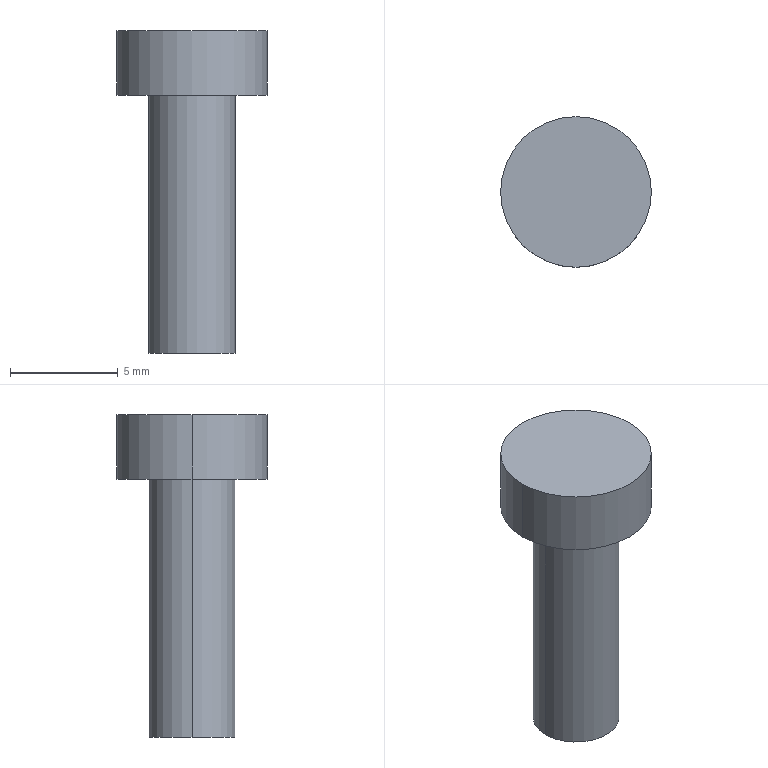Part | SolidWorks | features Extrusion 1, ICE 1 | 1 solid | 7 faces | box 7 x 7 x 15 mm | volume 266.25 mm3 | cylinder 4 | plane 3 | commonest cylinder face diameters 4 x2 7 x2
STEP:
#1=CARTESIAN_POINT('',(3.5,0.,3.));
#2=VERTEX_POINT('',#1);
#3=CARTESIAN_POINT('',(-3.5,0.,3.));
#4=VERTEX_POINT('',#3);
#5=CARTESIAN_POINT('',(0.,0.,3.));
#6=DIRECTION('',(0.,0.,1.));
#7=DIRECTION('',(1.,0.,0.));
#8=AXIS2_PLACEMENT_3D('',#5,#6,#7);
#9=CIRCLE('',#8,3.5);
#10=EDGE_CURVE('',#2,#4,#9,.T.);
#11=ORIENTED_EDGE('',*,*,#10,.F.);
#12=CARTESIAN_POINT('',(3.5,0.,0.));
#13=VERTEX_POINT('',#12);
#14=CARTESIAN_POINT('',(3.5,0.,3.));
#15=DIRECTION('',(0.,0.,-1.));
#16=VECTOR('',#15,1000.);
#17=LINE('',#14,#16);
#18=EDGE_CURVE('',#2,#13,#17,.T.);
#19=ORIENTED_EDGE('',*,*,#18,.T.);
#20=CARTESIAN_POINT('',(-3.5,0.,0.));
#21=VERTEX_POINT('',#20);
#22=CARTESIAN_POINT('',(0.,0.,0.));
#23=DIRECTION('',(0.,0.,1.));
#24=DIRECTION('',(1.,0.,0.));
#25=AXIS2_PLACEMENT_3D('',#22,#23,#24);
#26=CIRCLE('',#25,3.5);
#27=EDGE_CURVE('',#13,#21,#26,.T.);
#28=ORIENTED_EDGE('',*,*,#27,.T.);
#29=CARTESIAN_POINT('',(-3.5,0.,3.));
#30=DIRECTION('',(0.,0.,-1.));
#31=VECTOR('',#30,1000.);
#32=LINE('',#29,#31);
#33=EDGE_CURVE('',#4,#21,#32,.T.);
#34=ORIENTED_EDGE('',*,*,#33,.F.);
#35=EDGE_LOOP('',(#11,#19,#28,#34));
#36=FACE_OUTER_BOUND('',#35,.T.);
#37=CARTESIAN_POINT('',(0.,0.,3.));
#38=DIRECTION('',(0.,0.,-1.));
#39=DIRECTION('',(-1.,0.,0.));
#40=AXIS2_PLACEMENT_3D('',#37,#38,#39);
#41=CYLINDRICAL_SURFACE('',#40,3.5);
#42=ADVANCED_FACE('',(#36),#41,.T.);
#43=CARTESIAN_POINT('',(2.,0.,-12.));
#44=VERTEX_POINT('',#43);
#45=CARTESIAN_POINT('',(-2.,0.,-12.));
#46=VERTEX_POINT('',#45);
#47=CARTESIAN_POINT('',(0.,0.,-12.));
#48=DIRECTION('',(0.,0.,1.));
#49=DIRECTION('',(1.,0.,0.));
#50=AXIS2_PLACEMENT_3D('',#47,#48,#49);
#51=CIRCLE('',#50,2.);
#52=EDGE_CURVE('',#44,#46,#51,.T.);
#53=ORIENTED_EDGE('',*,*,#52,.T.);
#54=CARTESIAN_POINT('',(-2.,0.,0.));
#55=VERTEX_POINT('',#54);
#56=CARTESIAN_POINT('',(-2.,0.,-12.));
#57=DIRECTION('',(0.,0.,1.));
#58=VECTOR('',#57,1000.);
#59=LINE('',#56,#58);
#60=EDGE_CURVE('',#46,#55,#59,.T.);
#61=ORIENTED_EDGE('',*,*,#60,.T.);
#62=CARTESIAN_POINT('',(2.,0.,0.));
#63=VERTEX_POINT('',#62);
#64=CARTESIAN_POINT('',(0.,0.,0.));
#65=DIRECTION('',(0.,0.,1.));
#66=DIRECTION('',(1.,0.,0.));
#67=AXIS2_PLACEMENT_3D('',#64,#65,#66);
#68=CIRCLE('',#67,2.);
#69=EDGE_CURVE('',#63,#55,#68,.T.);
#70=ORIENTED_EDGE('',*,*,#69,.F.);
#71=CARTESIAN_POINT('',(2.,0.,-12.));
#72=DIRECTION('',(0.,0.,1.));
#73=VECTOR('',#72,1000.);
#74=LINE('',#71,#73);
#75=EDGE_CURVE('',#44,#63,#74,.T.);
#76=ORIENTED_EDGE('',*,*,#75,.F.);
#77=EDGE_LOOP('',(#53,#61,#70,#76));
#78=FACE_OUTER_BOUND('',#77,.T.);
#79=CARTESIAN_POINT('',(0.,0.,-12.));
#80=DIRECTION('',(0.,0.,1.));
#81=DIRECTION('',(1.,0.,0.));
#82=AXIS2_PLACEMENT_3D('',#79,#80,#81);
#83=CYLINDRICAL_SURFACE('',#82,2.);
#84=ADVANCED_FACE('',(#78),#83,.T.);
#85=ORIENTED_EDGE('',*,*,#60,.F.);
#86=CARTESIAN_POINT('',(0.,0.,-12.));
#87=DIRECTION('',(0.,0.,1.));
#88=DIRECTION('',(1.,0.,0.));
#89=AXIS2_PLACEMENT_3D('',#86,#87,#88);
#90=CIRCLE('',#89,2.);
#91=EDGE_CURVE('',#46,#44,#90,.T.);
#92=ORIENTED_EDGE('',*,*,#91,.T.);
#93=ORIENTED_EDGE('',*,*,#75,.T.);
#94=CARTESIAN_POINT('',(0.,0.,0.));
#95=DIRECTION('',(0.,0.,1.));
#96=DIRECTION('',(1.,0.,0.));
#97=AXIS2_PLACEMENT_3D('',#94,#95,#96);
#98=CIRCLE('',#97,2.);
#99=EDGE_CURVE('',#55,#63,#98,.T.);
#100=ORIENTED_EDGE('',*,*,#99,.F.);
#101=EDGE_LOOP('',(#85,#92,#93,#100));
#102=FACE_OUTER_BOUND('',#101,.T.);
#103=CARTESIAN_POINT('',(0.,0.,-12.));
#104=DIRECTION('',(0.,0.,1.));
#105=DIRECTION('',(1.,0.,0.));
#106=AXIS2_PLACEMENT_3D('',#103,#104,#105);
#107=CYLINDRICAL_SURFACE('',#106,2.);
#108=ADVANCED_FACE('',(#102),#107,.T.);
#109=ORIENTED_EDGE('',*,*,#52,.F.);
#110=ORIENTED_EDGE('',*,*,#91,.F.);
#111=EDGE_LOOP('',(#109,#110));
#112=FACE_OUTER_BOUND('',#111,.T.);
#113=CARTESIAN_POINT('',(0.,0.,-12.));
#114=DIRECTION('',(0.,0.,1.));
#115=DIRECTION('',(1.,0.,0.));
#116=AXIS2_PLACEMENT_3D('',#113,#114,#115);
#117=PLANE('',#116);
#118=ADVANCED_FACE('',(#112),#117,.F.);
#119=ORIENTED_EDGE('',*,*,#18,.F.);
#120=CARTESIAN_POINT('',(0.,0.,3.));
#121=DIRECTION('',(0.,0.,1.));
#122=DIRECTION('',(1.,0.,0.));
#123=AXIS2_PLACEMENT_3D('',#120,#121,#122);
#124=CIRCLE('',#123,3.5);
#125=EDGE_CURVE('',#4,#2,#124,.T.);
#126=ORIENTED_EDGE('',*,*,#125,.F.);
#127=ORIENTED_EDGE('',*,*,#33,.T.);
#128=CARTESIAN_POINT('',(0.,0.,0.));
#129=DIRECTION('',(0.,0.,1.));
#130=DIRECTION('',(1.,0.,0.));
#131=AXIS2_PLACEMENT_3D('',#128,#129,#130);
#132=CIRCLE('',#131,3.5);
#133=EDGE_CURVE('',#21,#13,#132,.T.);
#134=ORIENTED_EDGE('',*,*,#133,.T.);
#135=EDGE_LOOP('',(#119,#126,#127,#134));
#136=FACE_OUTER_BOUND('',#135,.T.);
#137=CARTESIAN_POINT('',(0.,0.,3.));
#138=DIRECTION('',(0.,0.,-1.));
#139=DIRECTION('',(-1.,0.,0.));
#140=AXIS2_PLACEMENT_3D('',#137,#138,#139);
#141=CYLINDRICAL_SURFACE('',#140,3.5);
#142=ADVANCED_FACE('',(#136),#141,.T.);
#143=ORIENTED_EDGE('',*,*,#125,.T.);
#144=ORIENTED_EDGE('',*,*,#10,.T.);
#145=EDGE_LOOP('',(#143,#144));
#146=FACE_OUTER_BOUND('',#145,.T.);
#147=CARTESIAN_POINT('',(0.,0.,3.));
#148=DIRECTION('',(0.,0.,1.));
#149=DIRECTION('',(1.,0.,0.));
#150=AXIS2_PLACEMENT_3D('',#147,#148,#149);
#151=PLANE('',#150);
#152=ADVANCED_FACE('',(#146),#151,.T.);
#153=ORIENTED_EDGE('',*,*,#69,.T.);
#154=ORIENTED_EDGE('',*,*,#99,.T.);
#155=EDGE_LOOP('',(#153,#154));
#156=FACE_BOUND('',#155,.T.);
#157=ORIENTED_EDGE('',*,*,#133,.F.);
#158=ORIENTED_EDGE('',*,*,#27,.F.);
#159=EDGE_LOOP('',(#157,#158));
#160=FACE_OUTER_BOUND('',#159,.T.);
#161=CARTESIAN_POINT('',(0.,0.,0.));
#162=DIRECTION('',(0.,0.,1.));
#163=DIRECTION('',(1.,0.,0.));
#164=AXIS2_PLACEMENT_3D('',#161,#162,#163);
#165=PLANE('',#164);
#166=ADVANCED_FACE('',(#156,#160),#165,.F.);
#167=CLOSED_SHELL('',(#42,#84,#108,#118,#142,#152,#166));
#168=MANIFOLD_SOLID_BREP('',#167);
#169=CARTESIAN_POINT('',(0.,0.,0.));
#170=DIRECTION('',(0.,0.,1.));
#171=DIRECTION('',(1.,0.,0.));
#172=AXIS2_PLACEMENT_3D('',#169,#170,#171);
#173=(LENGTH_UNIT()NAMED_UNIT(*)SI_UNIT(.MILLI.,.METRE.));
#174=UNCERTAINTY_MEASURE_WITH_UNIT(LENGTH_MEASURE(0.00001),#173,'','');
#175=(NAMED_UNIT(*)PLANE_ANGLE_UNIT()SI_UNIT($,.RADIAN.));
#176=(NAMED_UNIT(*)SI_UNIT($,.STERADIAN.)SOLID_ANGLE_UNIT());
#177=(GEOMETRIC_REPRESENTATION_CONTEXT(3)GLOBAL_UNCERTAINTY_ASSIGNED_CONTEXT((#174))GLOBAL_UNIT_ASSIGNED_CONTEXT((#173,#175,#176))REPRESENTATION_CONTEXT('',''));
#178=ADVANCED_BREP_SHAPE_REPRESENTATION('',(#168,#172),#177);